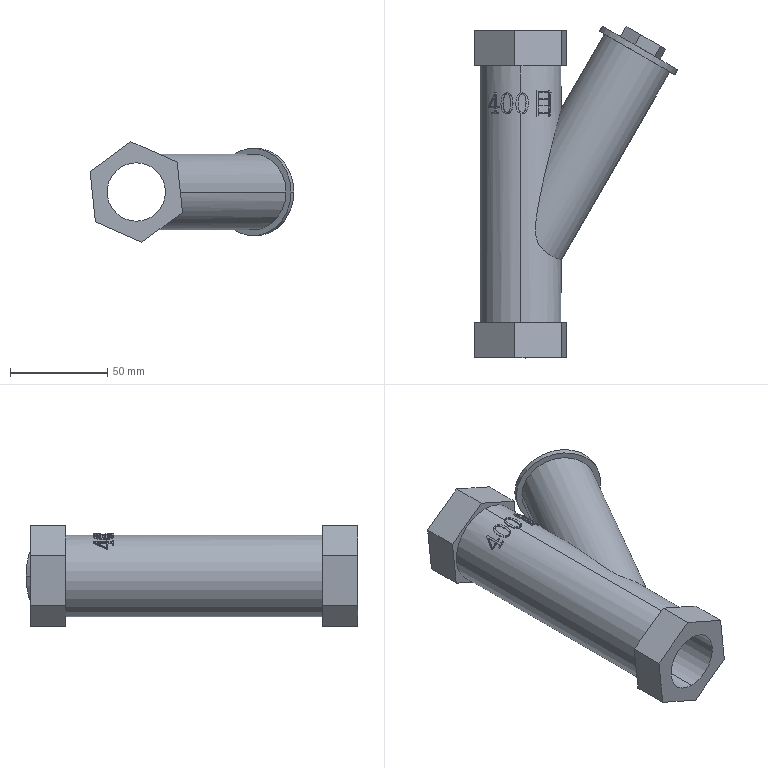Part | SolidWorks | features ICE 5, Emboss 1, Extrusion 1, Scale 1, Sweep 1 | 1 solid | 105 faces | box 104.725 x 170.486 x 51.675 mm | volume 233814 mm3 | spline 61 | plane 26 | cylinder 18 | commonest cylinder face diameters 42 x8 43.2 x4 30 x2 39 x2 45 x2